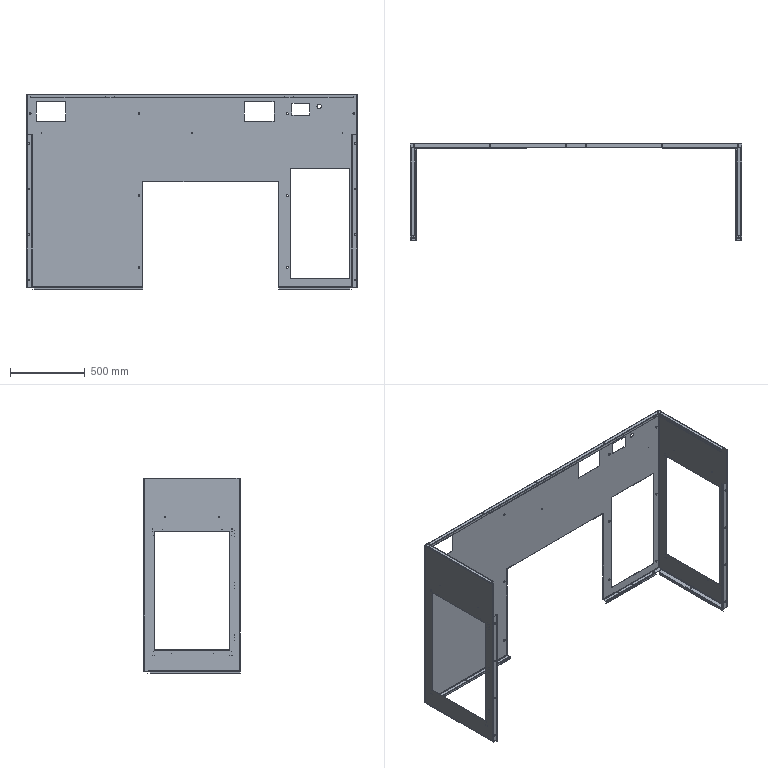Part | NX | features solid 2 | 1 solid | 388 faces | box 2220 x 650 x 1310 mm | volume 6196053 mm3 | cylinder 210 | plane 178 | commonest cylinder face diameters 1 x82 12 x40 4 x20 8 x20 10 x20 3 x14